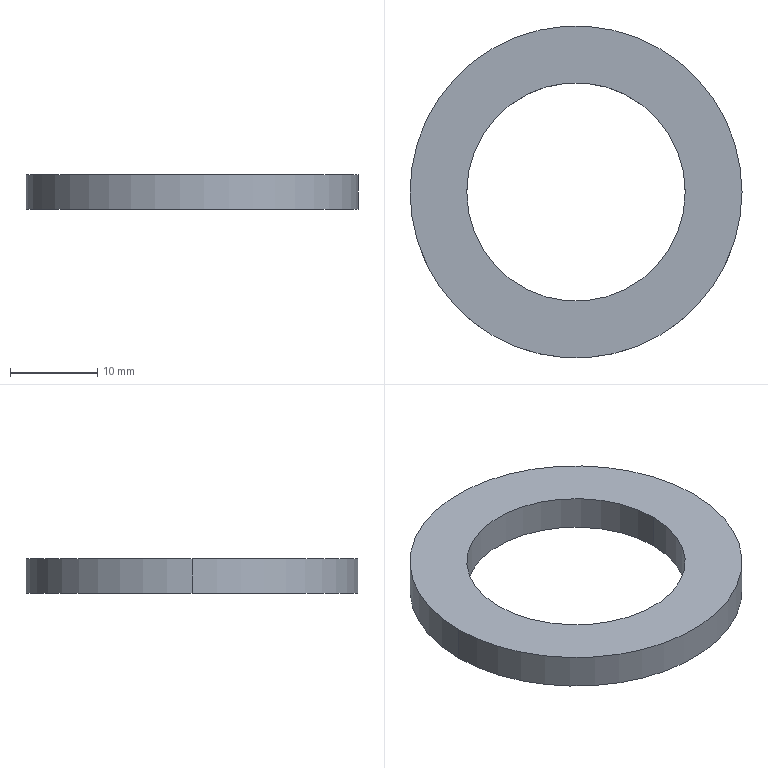Part | SolidWorks | features Extrusion 1 | 1 solid | 6 faces | box 38 x 38 x 4 mm | volume 2573 mm3 | cylinder 4 | plane 2 | commonest cylinder face diameters 25 x2 38 x2
STEP:
#1=CARTESIAN_POINT('',(-12.5,0.,4.));
#2=VERTEX_POINT('',#1);
#3=CARTESIAN_POINT('',(12.5,0.,4.));
#4=VERTEX_POINT('',#3);
#5=CARTESIAN_POINT('',(0.,0.,4.));
#6=DIRECTION('',(0.,0.,1.));
#7=DIRECTION('',(1.,0.,0.));
#8=AXIS2_PLACEMENT_3D('',#5,#6,#7);
#9=CIRCLE('',#8,12.5);
#10=EDGE_CURVE('',#2,#4,#9,.T.);
#11=ORIENTED_EDGE('',*,*,#10,.T.);
#12=CARTESIAN_POINT('',(12.5,0.,0.));
#13=VERTEX_POINT('',#12);
#14=CARTESIAN_POINT('',(12.5,0.,4.));
#15=DIRECTION('',(0.,0.,-1.));
#16=VECTOR('',#15,1000.);
#17=LINE('',#14,#16);
#18=EDGE_CURVE('',#4,#13,#17,.T.);
#19=ORIENTED_EDGE('',*,*,#18,.T.);
#20=CARTESIAN_POINT('',(-12.5,0.,0.));
#21=VERTEX_POINT('',#20);
#22=CARTESIAN_POINT('',(0.,0.,0.));
#23=DIRECTION('',(0.,0.,1.));
#24=DIRECTION('',(1.,0.,0.));
#25=AXIS2_PLACEMENT_3D('',#22,#23,#24);
#26=CIRCLE('',#25,12.5);
#27=EDGE_CURVE('',#21,#13,#26,.T.);
#28=ORIENTED_EDGE('',*,*,#27,.F.);
#29=CARTESIAN_POINT('',(-12.5,0.,4.));
#30=DIRECTION('',(0.,0.,-1.));
#31=VECTOR('',#30,1000.);
#32=LINE('',#29,#31);
#33=EDGE_CURVE('',#2,#21,#32,.T.);
#34=ORIENTED_EDGE('',*,*,#33,.F.);
#35=EDGE_LOOP('',(#11,#19,#28,#34));
#36=FACE_OUTER_BOUND('',#35,.T.);
#37=CARTESIAN_POINT('',(0.,0.,4.));
#38=DIRECTION('',(0.,0.,-1.));
#39=DIRECTION('',(-1.,0.,0.));
#40=AXIS2_PLACEMENT_3D('',#37,#38,#39);
#41=CYLINDRICAL_SURFACE('',#40,12.5);
#42=ADVANCED_FACE('',(#36),#41,.F.);
#43=CARTESIAN_POINT('',(19.,0.,4.));
#44=VERTEX_POINT('',#43);
#45=CARTESIAN_POINT('',(-19.,0.,4.));
#46=VERTEX_POINT('',#45);
#47=CARTESIAN_POINT('',(0.,0.,4.));
#48=DIRECTION('',(0.,0.,1.));
#49=DIRECTION('',(1.,0.,0.));
#50=AXIS2_PLACEMENT_3D('',#47,#48,#49);
#51=CIRCLE('',#50,19.);
#52=EDGE_CURVE('',#44,#46,#51,.T.);
#53=ORIENTED_EDGE('',*,*,#52,.F.);
#54=CARTESIAN_POINT('',(19.,0.,0.));
#55=VERTEX_POINT('',#54);
#56=CARTESIAN_POINT('',(19.,0.,4.));
#57=DIRECTION('',(0.,0.,-1.));
#58=VECTOR('',#57,1000.);
#59=LINE('',#56,#58);
#60=EDGE_CURVE('',#44,#55,#59,.T.);
#61=ORIENTED_EDGE('',*,*,#60,.T.);
#62=CARTESIAN_POINT('',(-19.,0.,0.));
#63=VERTEX_POINT('',#62);
#64=CARTESIAN_POINT('',(0.,0.,0.));
#65=DIRECTION('',(0.,0.,1.));
#66=DIRECTION('',(1.,0.,0.));
#67=AXIS2_PLACEMENT_3D('',#64,#65,#66);
#68=CIRCLE('',#67,19.);
#69=EDGE_CURVE('',#55,#63,#68,.T.);
#70=ORIENTED_EDGE('',*,*,#69,.T.);
#71=CARTESIAN_POINT('',(-19.,0.,4.));
#72=DIRECTION('',(0.,0.,-1.));
#73=VECTOR('',#72,1000.);
#74=LINE('',#71,#73);
#75=EDGE_CURVE('',#46,#63,#74,.T.);
#76=ORIENTED_EDGE('',*,*,#75,.F.);
#77=EDGE_LOOP('',(#53,#61,#70,#76));
#78=FACE_OUTER_BOUND('',#77,.T.);
#79=CARTESIAN_POINT('',(0.,0.,4.));
#80=DIRECTION('',(0.,0.,-1.));
#81=DIRECTION('',(-1.,0.,0.));
#82=AXIS2_PLACEMENT_3D('',#79,#80,#81);
#83=CYLINDRICAL_SURFACE('',#82,19.);
#84=ADVANCED_FACE('',(#78),#83,.T.);
#85=CARTESIAN_POINT('',(0.,0.,4.));
#86=DIRECTION('',(0.,0.,1.));
#87=DIRECTION('',(1.,0.,0.));
#88=AXIS2_PLACEMENT_3D('',#85,#86,#87);
#89=CIRCLE('',#88,19.);
#90=EDGE_CURVE('',#46,#44,#89,.T.);
#91=ORIENTED_EDGE('',*,*,#90,.T.);
#92=ORIENTED_EDGE('',*,*,#52,.T.);
#93=EDGE_LOOP('',(#91,#92));
#94=FACE_OUTER_BOUND('',#93,.T.);
#95=ORIENTED_EDGE('',*,*,#10,.F.);
#96=CARTESIAN_POINT('',(0.,0.,4.));
#97=DIRECTION('',(0.,0.,1.));
#98=DIRECTION('',(1.,0.,0.));
#99=AXIS2_PLACEMENT_3D('',#96,#97,#98);
#100=CIRCLE('',#99,12.5);
#101=EDGE_CURVE('',#4,#2,#100,.T.);
#102=ORIENTED_EDGE('',*,*,#101,.F.);
#103=EDGE_LOOP('',(#95,#102));
#104=FACE_BOUND('',#103,.T.);
#105=CARTESIAN_POINT('',(0.,0.,4.));
#106=DIRECTION('',(0.,0.,1.));
#107=DIRECTION('',(1.,0.,0.));
#108=AXIS2_PLACEMENT_3D('',#105,#106,#107);
#109=PLANE('',#108);
#110=ADVANCED_FACE('',(#94,#104),#109,.T.);
#111=CARTESIAN_POINT('',(0.,0.,0.));
#112=DIRECTION('',(0.,0.,1.));
#113=DIRECTION('',(1.,0.,0.));
#114=AXIS2_PLACEMENT_3D('',#111,#112,#113);
#115=CIRCLE('',#114,19.);
#116=EDGE_CURVE('',#63,#55,#115,.T.);
#117=ORIENTED_EDGE('',*,*,#116,.F.);
#118=ORIENTED_EDGE('',*,*,#69,.F.);
#119=EDGE_LOOP('',(#117,#118));
#120=FACE_OUTER_BOUND('',#119,.T.);
#121=ORIENTED_EDGE('',*,*,#27,.T.);
#122=CARTESIAN_POINT('',(0.,0.,0.));
#123=DIRECTION('',(0.,0.,1.));
#124=DIRECTION('',(1.,0.,0.));
#125=AXIS2_PLACEMENT_3D('',#122,#123,#124);
#126=CIRCLE('',#125,12.5);
#127=EDGE_CURVE('',#13,#21,#126,.T.);
#128=ORIENTED_EDGE('',*,*,#127,.T.);
#129=EDGE_LOOP('',(#121,#128));
#130=FACE_BOUND('',#129,.T.);
#131=CARTESIAN_POINT('',(0.,0.,0.));
#132=DIRECTION('',(0.,0.,1.));
#133=DIRECTION('',(1.,0.,0.));
#134=AXIS2_PLACEMENT_3D('',#131,#132,#133);
#135=PLANE('',#134);
#136=ADVANCED_FACE('',(#120,#130),#135,.F.);
#137=ORIENTED_EDGE('',*,*,#60,.F.);
#138=ORIENTED_EDGE('',*,*,#90,.F.);
#139=ORIENTED_EDGE('',*,*,#75,.T.);
#140=ORIENTED_EDGE('',*,*,#116,.T.);
#141=EDGE_LOOP('',(#137,#138,#139,#140));
#142=FACE_OUTER_BOUND('',#141,.T.);
#143=CARTESIAN_POINT('',(0.,0.,4.));
#144=DIRECTION('',(0.,0.,-1.));
#145=DIRECTION('',(-1.,0.,0.));
#146=AXIS2_PLACEMENT_3D('',#143,#144,#145);
#147=CYLINDRICAL_SURFACE('',#146,19.);
#148=ADVANCED_FACE('',(#142),#147,.T.);
#149=ORIENTED_EDGE('',*,*,#18,.F.);
#150=ORIENTED_EDGE('',*,*,#101,.T.);
#151=ORIENTED_EDGE('',*,*,#33,.T.);
#152=ORIENTED_EDGE('',*,*,#127,.F.);
#153=EDGE_LOOP('',(#149,#150,#151,#152));
#154=FACE_OUTER_BOUND('',#153,.T.);
#155=CARTESIAN_POINT('',(0.,0.,4.));
#156=DIRECTION('',(0.,0.,-1.));
#157=DIRECTION('',(-1.,0.,0.));
#158=AXIS2_PLACEMENT_3D('',#155,#156,#157);
#159=CYLINDRICAL_SURFACE('',#158,12.5);
#160=ADVANCED_FACE('',(#154),#159,.F.);
#161=CLOSED_SHELL('',(#42,#84,#110,#136,#148,#160));
#162=MANIFOLD_SOLID_BREP('',#161);
#163=CARTESIAN_POINT('',(0.,0.,0.));
#164=DIRECTION('',(0.,0.,1.));
#165=DIRECTION('',(1.,0.,0.));
#166=AXIS2_PLACEMENT_3D('',#163,#164,#165);
#167=(LENGTH_UNIT()NAMED_UNIT(*)SI_UNIT(.MILLI.,.METRE.));
#168=UNCERTAINTY_MEASURE_WITH_UNIT(LENGTH_MEASURE(0.00001),#167,'','');
#169=(NAMED_UNIT(*)PLANE_ANGLE_UNIT()SI_UNIT($,.RADIAN.));
#170=(NAMED_UNIT(*)SI_UNIT($,.STERADIAN.)SOLID_ANGLE_UNIT());
#171=(GEOMETRIC_REPRESENTATION_CONTEXT(3)GLOBAL_UNCERTAINTY_ASSIGNED_CONTEXT((#168))GLOBAL_UNIT_ASSIGNED_CONTEXT((#167,#169,#170))REPRESENTATION_CONTEXT('',''));
#172=ADVANCED_BREP_SHAPE_REPRESENTATION('',(#162,#166),#171);